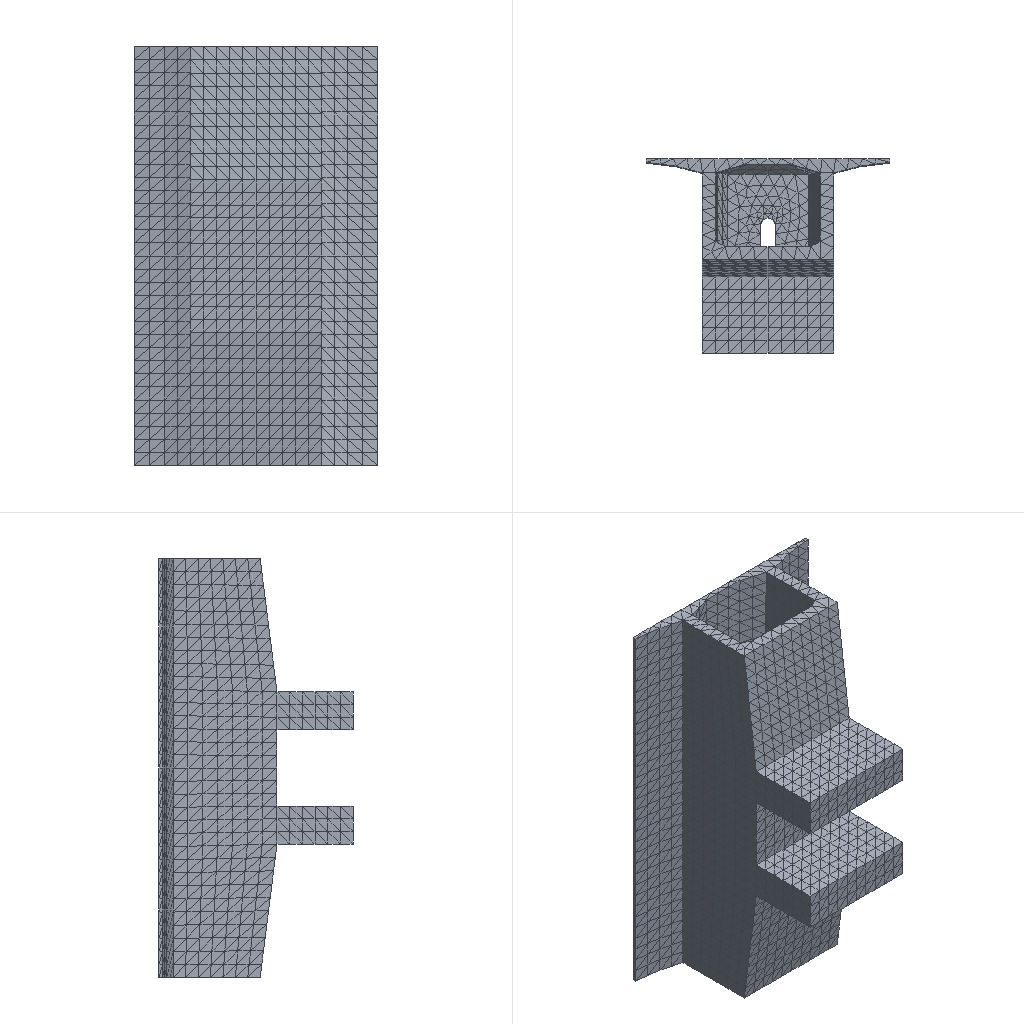Simulation study | abaqus
Set-up summary:
category,name,step,type,value,unit,region
solver,abaqus
solver,version,,,Abaqus/Standard 2020
units,not stated in the deck,,not stated
analysis,deck,,static,static
load_step,Step-1,Step-1,static,nlgeom=True
contact,interactions,,,general=0 pairs=0 ties=0
load_step,requested,,,1
mesh,nodes,,,13119
mesh,elements,,,22370
element_type,C3D4,,solid,18115
element_type,T3D2,,truss,4255
load,load commands in deck,,count,4
bc,support commands in deck,,count,1
material,C40,,in results
material,FIBER,,in results
check,setup vs results,,match,"per instance, exact: element labels, types and connectivity; labels of the nodes the elements use; coordinates of those nodes at SINGLE_PRECISION in 6 of 6 instance(s)"
Results summary:
result,step,,completed,increments=12 time=1.0/1.0
result,analysis,,,static
result,last_loadstep,,,1
result,analysis steps,,count,1
result,primary field,,,U
result,reaction total,,FX,-0.016,model units
result,reaction total,,FY,199980.734,model units
result,reaction total,,FZ,0.08621,model units